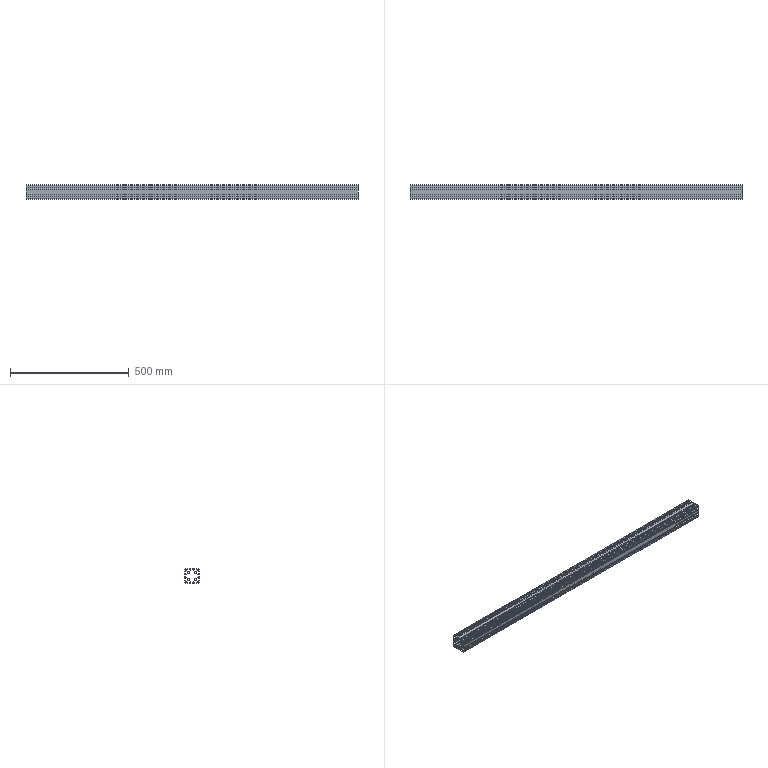Part | STEP file | 2_Default <Machined> | 1 solid | 178 faces | box 1400 x 60 x 60 mm | volume 1288545 mm3 | plane 162 | cylinder 16 | commonest cylinder face diameters 6.8 x8 6.76 x4 11.828 x4